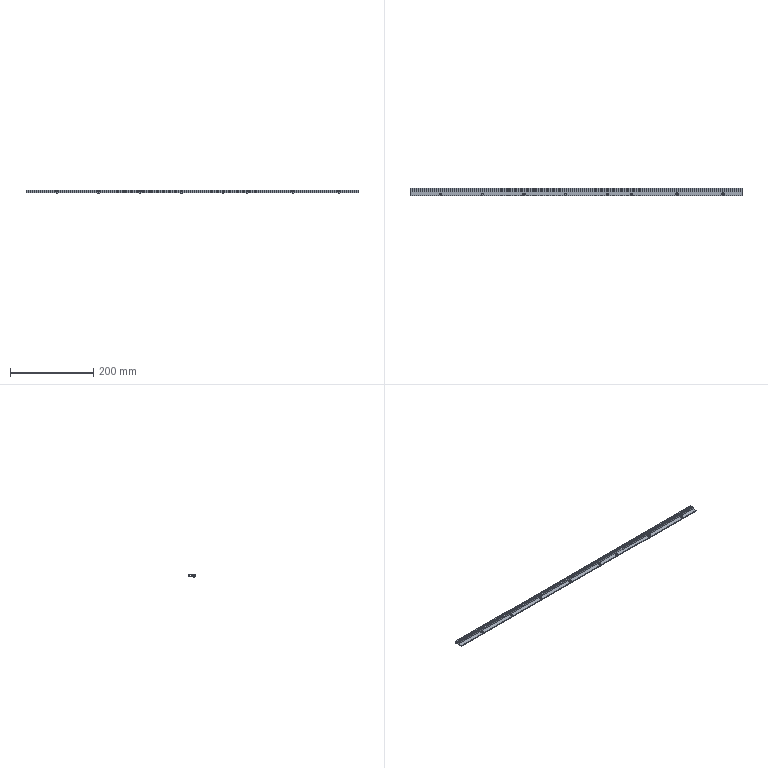Part | STEP file | Guide wheel mechanism revised.sldasm-Part-413 | 1 solid | 238 faces | box 798 x 19 x 9 mm | volume 44595 mm3 | cone 108 | plane 68 | cylinder 62 | commonest cylinder face diameters 5.765 x46 3 x16